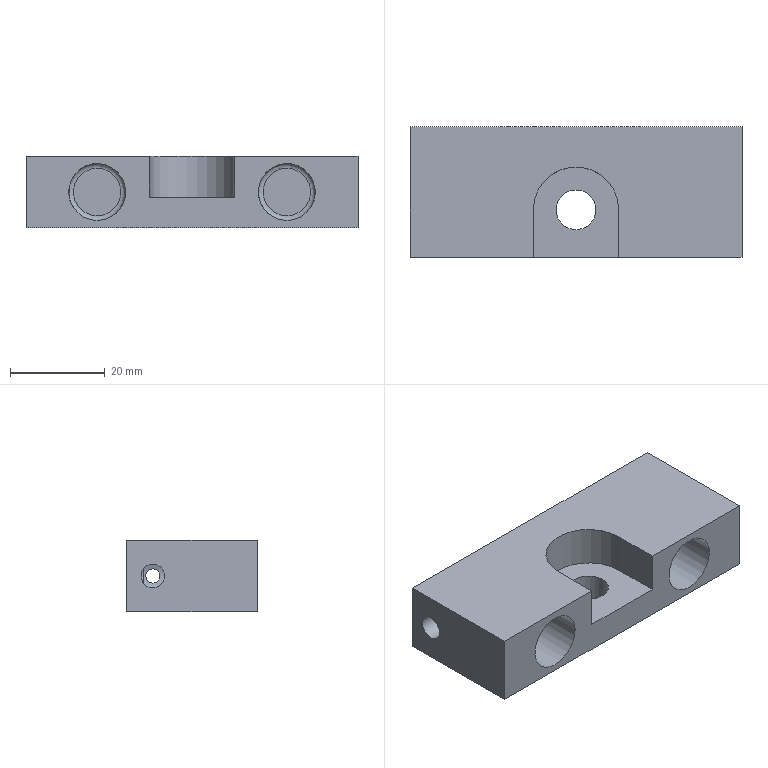Part | NX | 1 solid | 20 faces | box 70 x 27.5 x 15 mm | volume 19680 mm3 | plane 11 | cylinder 7 | torus 2 | commonest cylinder face diameters 5 x2 12 x2 3 x1 8.4 x1 18 x1
STEP:
#1=CARTESIAN_POINT('',(-25.809,10.25,-6.));
#2=VERTEX_POINT('',#1);
#3=CARTESIAN_POINT('',(-25.809,10.25,-9.));
#4=VERTEX_POINT('',#3);
#5=CARTESIAN_POINT('',(-25.809,10.25,-9.));
#6=CARTESIAN_POINT('',(-25.835,10.323,-8.902));
#7=CARTESIAN_POINT('',(-25.863,10.446,-8.704));
#8=CARTESIAN_POINT('',(-25.873,10.542,-8.508));
#9=CARTESIAN_POINT('',(-25.876,10.631,-8.268));
#10=CARTESIAN_POINT('',(-25.875,10.659,-8.178));
#11=CARTESIAN_POINT('',(-25.868,10.746,-7.791));
#12=CARTESIAN_POINT('',(-25.864,10.753,-7.504));
#13=CARTESIAN_POINT('',(-25.868,10.746,-7.206));
#14=CARTESIAN_POINT('',(-25.875,10.66,-6.826));
#15=CARTESIAN_POINT('',(-25.876,10.632,-6.733));
#16=CARTESIAN_POINT('',(-25.873,10.541,-6.491));
#17=CARTESIAN_POINT('',(-25.862,10.444,-6.293));
#18=CARTESIAN_POINT('',(-25.835,10.323,-6.098));
#19=CARTESIAN_POINT('',(-25.809,10.25,-6.));
#20=B_SPLINE_CURVE_WITH_KNOTS('',3,(#5,#6,#7,#8,#9,#10,#11,#12,#13,#14,#15,#16,#17,#18,#19),.UNSPECIFIED.,.F.,.F.,(4,1,1,1,1,1,1,1,1,1,1,1,4),(0.,0.125,0.1875,0.25,0.3125,0.375,0.5,0.625,0.6875,0.75,0.8125,0.875,1.),.UNSPECIFIED.);
#21=EDGE_CURVE('',#2,#4,#20,.F.);
#22=ORIENTED_EDGE('',*,*,#21,.F.);
#23=CARTESIAN_POINT('',(-25.809,10.25,-6.));
#24=CARTESIAN_POINT('',(-25.79,10.195,-5.926));
#25=CARTESIAN_POINT('',(-25.746,10.067,-5.766));
#26=CARTESIAN_POINT('',(-25.671,9.804,-5.539));
#27=CARTESIAN_POINT('',(-25.638,9.681,-5.445));
#28=CARTESIAN_POINT('',(-25.553,9.31,-5.222));
#29=CARTESIAN_POINT('',(-25.488,8.921,-5.075));
#30=CARTESIAN_POINT('',(-25.444,8.343,-4.977));
#31=CARTESIAN_POINT('',(-25.465,7.851,-5.021));
#32=CARTESIAN_POINT('',(-25.511,7.433,-5.127));
#33=CARTESIAN_POINT('',(-25.556,7.185,-5.234));
#34=CARTESIAN_POINT('',(-25.605,6.955,-5.356));
#35=CARTESIAN_POINT('',(-25.659,6.74,-5.506));
#36=CARTESIAN_POINT('',(-25.675,6.681,-5.549));
#37=CARTESIAN_POINT('',(-25.762,6.385,-5.817));
#38=CARTESIAN_POINT('',(-25.814,6.235,-6.008));
#39=CARTESIAN_POINT('',(-25.903,5.99,-6.404));
#40=CARTESIAN_POINT('',(-25.969,5.826,-6.822));
#41=CARTESIAN_POINT('',(-26.021,5.698,-7.504));
#42=CARTESIAN_POINT('',(-25.968,5.828,-8.185));
#43=CARTESIAN_POINT('',(-25.902,5.992,-8.602));
#44=CARTESIAN_POINT('',(-25.813,6.238,-8.997));
#45=CARTESIAN_POINT('',(-25.761,6.388,-9.186));
#46=CARTESIAN_POINT('',(-25.675,6.682,-9.451));
#47=CARTESIAN_POINT('',(-25.658,6.745,-9.498));
#48=CARTESIAN_POINT('',(-25.604,6.959,-9.646));
#49=CARTESIAN_POINT('',(-25.556,7.188,-9.768));
#50=CARTESIAN_POINT('',(-25.491,7.552,-9.921));
#51=CARTESIAN_POINT('',(-25.431,8.229,-10.052));
#52=CARTESIAN_POINT('',(-25.489,8.924,-9.922));
#53=CARTESIAN_POINT('',(-25.553,9.314,-9.777));
#54=CARTESIAN_POINT('',(-25.638,9.684,-9.553));
#55=CARTESIAN_POINT('',(-25.671,9.806,-9.46));
#56=CARTESIAN_POINT('',(-25.747,10.069,-9.231));
#57=CARTESIAN_POINT('',(-25.79,10.195,-9.074));
#58=CARTESIAN_POINT('',(-25.809,10.25,-9.));
#59=B_SPLINE_CURVE_WITH_KNOTS('',3,(#23,#24,#25,#26,#27,#28,#29,#30,#31,#32,#33,#34,#35,#36,#37,#38,#39,#40,#41,#42,#43,#44,#45,#46,#47,#48,#49,#50,#51,#52,#53,#54,#55,#56,#57,#58),.UNSPECIFIED.,.F.,.F.,(4,1,1,1,1,1,1,1,1,1,1,1,1,1,1,1,1,1,1,1,1,1,1,1,1,1,1,1,1,1,1,1,1,4),(0.,0.03125,0.04688,0.0625,0.09375,0.125,0.1875,0.2188,0.25,0.2812,0.2969,0.3125,0.3281,0.3438,0.375,0.4062,0.4375,0.5,0.5625,0.5938,0.625,0.6562,0.6719,0.6875,0.7031,0.7188,0.75,0.8125,0.875,0.9062,0.9375,0.9531,0.9688,1.),.UNSPECIFIED.);
#60=EDGE_CURVE('',#4,#2,#59,.F.);
#61=ORIENTED_EDGE('',*,*,#60,.F.);
#62=EDGE_LOOP('',(#22,#61));
#63=FACE_BOUND('',#62,.T.);
#64=CARTESIAN_POINT('',(-35.,5.75,-7.5));
#65=VERTEX_POINT('',#64);
#66=CARTESIAN_POINT('',(-35.,8.25,-7.5));
#67=DIRECTION('',(-1.,0.,0.));
#68=DIRECTION('',(0.,-1.,0.));
#69=AXIS2_PLACEMENT_3D('',#66,#67,#68);
#70=CIRCLE('',#69,2.5);
#71=EDGE_CURVE('',#65,#65,#70,.T.);
#72=ORIENTED_EDGE('',*,*,#71,.T.);
#73=EDGE_LOOP('',(#72));
#74=FACE_BOUND('',#73,.T.);
#75=CARTESIAN_POINT('',(-20.,8.25,-7.5));
#76=DIRECTION('',(-1.,0.,0.));
#77=DIRECTION('',(0.,0.,1.));
#78=AXIS2_PLACEMENT_3D('',#75,#76,#77);
#79=CYLINDRICAL_SURFACE('',#78,2.5);
#80=ADVANCED_FACE('',(#63,#74),#79,.F.);
#81=CARTESIAN_POINT('',(-14.191,8.25,-9.));
#82=VERTEX_POINT('',#81);
#83=CARTESIAN_POINT('',(-14.169,8.786,-8.915));
#84=CARTESIAN_POINT('',(-14.204,8.276,-9.053));
#85=CARTESIAN_POINT('',(-14.172,7.744,-8.926));
#86=CARTESIAN_POINT('',(-14.143,7.499,-8.807));
#87=CARTESIAN_POINT('',(-14.1,7.208,-8.604));
#88=CARTESIAN_POINT('',(-14.053,6.973,-8.305));
#89=CARTESIAN_POINT('',(-14.021,6.837,-8.041));
#90=CARTESIAN_POINT('',(-13.987,6.699,-7.532));
#91=CARTESIAN_POINT('',(-14.017,6.818,-7.007));
#92=CARTESIAN_POINT('',(-14.047,6.947,-6.743));
#93=CARTESIAN_POINT('',(-14.088,7.144,-6.46));
#94=CARTESIAN_POINT('',(-14.137,7.451,-6.219));
#95=CARTESIAN_POINT('',(-14.168,7.708,-6.088));
#96=CARTESIAN_POINT('',(-14.204,8.218,-5.948));
#97=CARTESIAN_POINT('',(-14.173,8.745,-6.07));
#98=CARTESIAN_POINT('',(-14.143,9.,-6.192));
#99=CARTESIAN_POINT('',(-14.1,9.291,-6.395));
#100=CARTESIAN_POINT('',(-14.053,9.526,-6.694));
#101=CARTESIAN_POINT('',(-14.021,9.663,-6.96));
#102=CARTESIAN_POINT('',(-13.988,9.801,-7.468));
#103=CARTESIAN_POINT('',(-14.017,9.682,-7.992));
#104=CARTESIAN_POINT('',(-14.047,9.553,-8.257));
#105=CARTESIAN_POINT('',(-14.088,9.357,-8.539));
#106=CARTESIAN_POINT('',(-14.137,9.05,-8.781));
#107=CARTESIAN_POINT('',(-14.169,8.786,-8.915));
#108=CARTESIAN_POINT('',(-14.204,8.276,-9.053));
#109=CARTESIAN_POINT('',(-14.172,7.744,-8.926));
#110=B_SPLINE_CURVE_WITH_KNOTS('',3,(#83,#84,#85,#86,#87,#88,#89,#90,#91,#92,#93,#94,#95,#96,#97,#98,#99,#100,#101,#102,#103,#104,#105,#106,#107,#108,#109),.UNSPECIFIED.,.T.,.F.,(1,1,1,1,1,1,1,1,1,1,1,1,1,1,1,1,1,1,1,1,1,1,1,1,1,1,1,1,1,1,1),(-0.1283,-0.09704,-0.06579,0.,0.05937,0.09055,0.1217,0.153,0.1842,0.2467,0.3092,0.3405,0.3717,0.403,0.4342,0.4967,0.5592,0.5905,0.6217,0.653,0.6842,0.7467,0.8092,0.8405,0.8717,0.903,0.9342,1.,1.059,1.091,1.122),.UNSPECIFIED.);
#111=EDGE_CURVE('',#82,#82,#110,.F.);
#112=ORIENTED_EDGE('',*,*,#111,.F.);
#113=EDGE_LOOP('',(#112));
#114=FACE_BOUND('',#113,.T.);
#115=CARTESIAN_POINT('',(14.191,8.25,-9.));
#116=VERTEX_POINT('',#115);
#117=CARTESIAN_POINT('',(14.169,7.714,-8.915));
#118=CARTESIAN_POINT('',(14.204,8.224,-9.053));
#119=CARTESIAN_POINT('',(14.172,8.756,-8.926));
#120=CARTESIAN_POINT('',(14.143,9.001,-8.807));
#121=CARTESIAN_POINT('',(14.1,9.292,-8.604));
#122=CARTESIAN_POINT('',(14.053,9.527,-8.305));
#123=CARTESIAN_POINT('',(14.021,9.663,-8.041));
#124=CARTESIAN_POINT('',(13.987,9.801,-7.532));
#125=CARTESIAN_POINT('',(14.017,9.682,-7.007));
#126=CARTESIAN_POINT('',(14.047,9.553,-6.743));
#127=CARTESIAN_POINT('',(14.088,9.356,-6.46));
#128=CARTESIAN_POINT('',(14.137,9.049,-6.219));
#129=CARTESIAN_POINT('',(14.168,8.792,-6.088));
#130=CARTESIAN_POINT('',(14.204,8.282,-5.948));
#131=CARTESIAN_POINT('',(14.173,7.755,-6.07));
#132=CARTESIAN_POINT('',(14.143,7.5,-6.192));
#133=CARTESIAN_POINT('',(14.1,7.209,-6.395));
#134=CARTESIAN_POINT('',(14.053,6.974,-6.694));
#135=CARTESIAN_POINT('',(14.021,6.837,-6.96));
#136=CARTESIAN_POINT('',(13.988,6.699,-7.468));
#137=CARTESIAN_POINT('',(14.017,6.818,-7.992));
#138=CARTESIAN_POINT('',(14.047,6.947,-8.257));
#139=CARTESIAN_POINT('',(14.088,7.143,-8.539));
#140=CARTESIAN_POINT('',(14.137,7.45,-8.781));
#141=CARTESIAN_POINT('',(14.169,7.714,-8.915));
#142=CARTESIAN_POINT('',(14.204,8.224,-9.053));
#143=CARTESIAN_POINT('',(14.172,8.756,-8.926));
#144=B_SPLINE_CURVE_WITH_KNOTS('',3,(#117,#118,#119,#120,#121,#122,#123,#124,#125,#126,#127,#128,#129,#130,#131,#132,#133,#134,#135,#136,#137,#138,#139,#140,#141,#142,#143),.UNSPECIFIED.,.T.,.F.,(1,1,1,1,1,1,1,1,1,1,1,1,1,1,1,1,1,1,1,1,1,1,1,1,1,1,1,1,1,1,1),(-0.1283,-0.09704,-0.06579,0.,0.05937,0.09055,0.1217,0.153,0.1842,0.2467,0.3092,0.3405,0.3717,0.403,0.4342,0.4967,0.5592,0.5905,0.6217,0.653,0.6842,0.7467,0.8092,0.8405,0.8717,0.903,0.9342,1.,1.059,1.091,1.122),.UNSPECIFIED.);
#145=EDGE_CURVE('',#116,#116,#144,.F.);
#146=ORIENTED_EDGE('',*,*,#145,.F.);
#147=EDGE_LOOP('',(#146));
#148=FACE_BOUND('',#147,.T.);
#149=CARTESIAN_POINT('',(-20.,8.25,-7.5));
#150=DIRECTION('',(1.,0.,0.));
#151=DIRECTION('',(0.,0.,-1.));
#152=AXIS2_PLACEMENT_3D('',#149,#150,#151);
#153=CYLINDRICAL_SURFACE('',#152,1.5);
#154=ADVANCED_FACE('',(#114,#148),#153,.F.);
#155=CARTESIAN_POINT('',(25.809,10.25,-9.));
#156=VERTEX_POINT('',#155);
#157=CARTESIAN_POINT('',(25.809,10.25,-6.));
#158=VERTEX_POINT('',#157);
#159=CARTESIAN_POINT('',(25.809,10.25,-6.));
#160=CARTESIAN_POINT('',(25.835,10.323,-6.098));
#161=CARTESIAN_POINT('',(25.863,10.446,-6.296));
#162=CARTESIAN_POINT('',(25.873,10.542,-6.492));
#163=CARTESIAN_POINT('',(25.876,10.631,-6.732));
#164=CARTESIAN_POINT('',(25.875,10.659,-6.822));
#165=CARTESIAN_POINT('',(25.868,10.746,-7.209));
#166=CARTESIAN_POINT('',(25.864,10.753,-7.496));
#167=CARTESIAN_POINT('',(25.868,10.746,-7.794));
#168=CARTESIAN_POINT('',(25.875,10.66,-8.174));
#169=CARTESIAN_POINT('',(25.876,10.632,-8.267));
#170=CARTESIAN_POINT('',(25.873,10.541,-8.509));
#171=CARTESIAN_POINT('',(25.862,10.444,-8.707));
#172=CARTESIAN_POINT('',(25.835,10.323,-8.902));
#173=CARTESIAN_POINT('',(25.809,10.25,-9.));
#174=B_SPLINE_CURVE_WITH_KNOTS('',3,(#159,#160,#161,#162,#163,#164,#165,#166,#167,#168,#169,#170,#171,#172,#173),.UNSPECIFIED.,.F.,.F.,(4,1,1,1,1,1,1,1,1,1,1,1,4),(0.,0.125,0.1875,0.25,0.3125,0.375,0.5,0.625,0.6875,0.75,0.8125,0.875,1.),.UNSPECIFIED.);
#175=EDGE_CURVE('',#156,#158,#174,.F.);
#176=ORIENTED_EDGE('',*,*,#175,.F.);
#177=CARTESIAN_POINT('',(25.809,10.25,-9.));
#178=CARTESIAN_POINT('',(25.79,10.195,-9.074));
#179=CARTESIAN_POINT('',(25.746,10.067,-9.234));
#180=CARTESIAN_POINT('',(25.671,9.804,-9.461));
#181=CARTESIAN_POINT('',(25.638,9.681,-9.555));
#182=CARTESIAN_POINT('',(25.553,9.31,-9.778));
#183=CARTESIAN_POINT('',(25.488,8.921,-9.925));
#184=CARTESIAN_POINT('',(25.444,8.343,-10.023));
#185=CARTESIAN_POINT('',(25.465,7.851,-9.979));
#186=CARTESIAN_POINT('',(25.511,7.433,-9.873));
#187=CARTESIAN_POINT('',(25.556,7.185,-9.766));
#188=CARTESIAN_POINT('',(25.605,6.955,-9.644));
#189=CARTESIAN_POINT('',(25.659,6.74,-9.494));
#190=CARTESIAN_POINT('',(25.675,6.681,-9.451));
#191=CARTESIAN_POINT('',(25.762,6.385,-9.183));
#192=CARTESIAN_POINT('',(25.814,6.235,-8.992));
#193=CARTESIAN_POINT('',(25.903,5.99,-8.596));
#194=CARTESIAN_POINT('',(25.969,5.826,-8.178));
#195=CARTESIAN_POINT('',(26.021,5.698,-7.496));
#196=CARTESIAN_POINT('',(25.968,5.828,-6.815));
#197=CARTESIAN_POINT('',(25.902,5.992,-6.398));
#198=CARTESIAN_POINT('',(25.813,6.238,-6.003));
#199=CARTESIAN_POINT('',(25.761,6.388,-5.814));
#200=CARTESIAN_POINT('',(25.675,6.682,-5.549));
#201=CARTESIAN_POINT('',(25.658,6.745,-5.502));
#202=CARTESIAN_POINT('',(25.604,6.959,-5.354));
#203=CARTESIAN_POINT('',(25.556,7.188,-5.232));
#204=CARTESIAN_POINT('',(25.491,7.552,-5.079));
#205=CARTESIAN_POINT('',(25.431,8.229,-4.948));
#206=CARTESIAN_POINT('',(25.489,8.924,-5.078));
#207=CARTESIAN_POINT('',(25.553,9.314,-5.223));
#208=CARTESIAN_POINT('',(25.638,9.684,-5.447));
#209=CARTESIAN_POINT('',(25.671,9.806,-5.54));
#210=CARTESIAN_POINT('',(25.747,10.069,-5.769));
#211=CARTESIAN_POINT('',(25.79,10.195,-5.926));
#212=CARTESIAN_POINT('',(25.809,10.25,-6.));
#213=B_SPLINE_CURVE_WITH_KNOTS('',3,(#177,#178,#179,#180,#181,#182,#183,#184,#185,#186,#187,#188,#189,#190,#191,#192,#193,#194,#195,#196,#197,#198,#199,#200,#201,#202,#203,#204,#205,#206,#207,#208,#209,#210,#211,#212),.UNSPECIFIED.,.F.,.F.,(4,1,1,1,1,1,1,1,1,1,1,1,1,1,1,1,1,1,1,1,1,1,1,1,1,1,1,1,1,1,1,1,1,4),(0.,0.03125,0.04688,0.0625,0.09375,0.125,0.1875,0.2188,0.25,0.2812,0.2969,0.3125,0.3281,0.3438,0.375,0.4062,0.4375,0.5,0.5625,0.5938,0.625,0.6562,0.6719,0.6875,0.7031,0.7188,0.75,0.8125,0.875,0.9062,0.9375,0.9531,0.9688,1.),.UNSPECIFIED.);
#214=EDGE_CURVE('',#158,#156,#213,.F.);
#215=ORIENTED_EDGE('',*,*,#214,.F.);
#216=EDGE_LOOP('',(#176,#215));
#217=FACE_BOUND('',#216,.T.);
#218=CARTESIAN_POINT('',(35.,10.75,-7.5));
#219=VERTEX_POINT('',#218);
#220=CARTESIAN_POINT('',(35.,8.25,-7.5));
#221=DIRECTION('',(1.,0.,0.));
#222=DIRECTION('',(0.,1.,0.));
#223=AXIS2_PLACEMENT_3D('',#220,#221,#222);
#224=CIRCLE('',#223,2.5);
#225=EDGE_CURVE('',#219,#219,#224,.T.);
#226=ORIENTED_EDGE('',*,*,#225,.T.);
#227=EDGE_LOOP('',(#226));
#228=FACE_BOUND('',#227,.T.);
#229=CARTESIAN_POINT('',(20.,8.25,-7.5));
#230=DIRECTION('',(1.,0.,0.));
#231=DIRECTION('',(0.,0.,-1.));
#232=AXIS2_PLACEMENT_3D('',#229,#230,#231);
#233=CYLINDRICAL_SURFACE('',#232,2.5);
#234=ADVANCED_FACE('',(#217,#228),#233,.F.);
#235=CARTESIAN_POINT('',(-20.,11.25,-12.5));
#236=VERTEX_POINT('',#235);
#237=CARTESIAN_POINT('',(-20.,11.25,-7.5));
#238=DIRECTION('',(0.,-1.,0.));
#239=DIRECTION('',(0.,0.,-1.));
#240=AXIS2_PLACEMENT_3D('',#237,#238,#239);
#241=CIRCLE('',#240,5.);
#242=EDGE_CURVE('',#236,#236,#241,.T.);
#243=ORIENTED_EDGE('',*,*,#242,.F.);
#244=EDGE_LOOP('',(#243));
#245=FACE_BOUND('',#244,.T.);
#246=CARTESIAN_POINT('',(-20.,10.25,-7.5));
#247=DIRECTION('',(0.,-1.,0.));
#248=DIRECTION('',(0.,0.,-1.));
#249=AXIS2_PLACEMENT_3D('',#246,#247,#248);
#250=CIRCLE('',#249,6.);
#251=EDGE_CURVE('',#4,#2,#250,.T.);
#252=ORIENTED_EDGE('',*,*,#251,.T.);
#253=ORIENTED_EDGE('',*,*,#21,.T.);
#254=EDGE_LOOP('',(#252,#253));
#255=FACE_BOUND('',#254,.T.);
#256=CARTESIAN_POINT('',(-20.,10.25,-7.5));
#257=DIRECTION('',(0.,-1.,0.));
#258=DIRECTION('',(0.,0.,-1.));
#259=AXIS2_PLACEMENT_3D('',#256,#257,#258);
#260=TOROIDAL_SURFACE('',#259,5.,1.);
#261=ADVANCED_FACE('',(#245,#255),#260,.F.);
#262=CARTESIAN_POINT('',(20.,11.25,-12.5));
#263=VERTEX_POINT('',#262);
#264=CARTESIAN_POINT('',(20.,11.25,-7.5));
#265=DIRECTION('',(0.,-1.,0.));
#266=DIRECTION('',(0.,0.,-1.));
#267=AXIS2_PLACEMENT_3D('',#264,#265,#266);
#268=CIRCLE('',#267,5.);
#269=EDGE_CURVE('',#263,#263,#268,.T.);
#270=ORIENTED_EDGE('',*,*,#269,.F.);
#271=EDGE_LOOP('',(#270));
#272=FACE_BOUND('',#271,.T.);
#273=CARTESIAN_POINT('',(20.,10.25,-7.5));
#274=DIRECTION('',(0.,-1.,0.));
#275=DIRECTION('',(0.,0.,-1.));
#276=AXIS2_PLACEMENT_3D('',#273,#274,#275);
#277=CIRCLE('',#276,6.);
#278=EDGE_CURVE('',#158,#156,#277,.T.);
#279=ORIENTED_EDGE('',*,*,#278,.T.);
#280=ORIENTED_EDGE('',*,*,#175,.T.);
#281=EDGE_LOOP('',(#279,#280));
#282=FACE_BOUND('',#281,.T.);
#283=CARTESIAN_POINT('',(20.,10.25,-7.5));
#284=DIRECTION('',(0.,-1.,0.));
#285=DIRECTION('',(0.,0.,-1.));
#286=AXIS2_PLACEMENT_3D('',#283,#284,#285);
#287=TOROIDAL_SURFACE('',#286,5.,1.);
#288=ADVANCED_FACE('',(#272,#282),#287,.F.);
#289=ORIENTED_EDGE('',*,*,#269,.T.);
#290=EDGE_LOOP('',(#289));
#291=FACE_BOUND('',#290,.T.);
#292=CARTESIAN_POINT('',(20.,11.25,-7.5));
#293=DIRECTION('',(0.,-1.,0.));
#294=DIRECTION('',(0.,0.,-1.));
#295=AXIS2_PLACEMENT_3D('',#292,#293,#294);
#296=PLANE('',#295);
#297=ADVANCED_FACE('',(#291),#296,.T.);
#298=ORIENTED_EDGE('',*,*,#145,.T.);
#299=EDGE_LOOP('',(#298));
#300=FACE_BOUND('',#299,.T.);
#301=CARTESIAN_POINT('',(14.,-13.75,-7.5));
#302=VERTEX_POINT('',#301);
#303=CARTESIAN_POINT('',(20.,-13.75,-7.5));
#304=DIRECTION('',(0.,1.,0.));
#305=DIRECTION('',(-1.,0.,0.));
#306=AXIS2_PLACEMENT_3D('',#303,#304,#305);
#307=CIRCLE('',#306,6.);
#308=EDGE_CURVE('',#302,#302,#307,.F.);
#309=ORIENTED_EDGE('',*,*,#308,.T.);
#310=EDGE_LOOP('',(#309));
#311=FACE_BOUND('',#310,.T.);
#312=ORIENTED_EDGE('',*,*,#278,.F.);
#313=ORIENTED_EDGE('',*,*,#214,.T.);
#314=EDGE_LOOP('',(#312,#313));
#315=FACE_BOUND('',#314,.T.);
#316=CARTESIAN_POINT('',(20.,11.25,-7.5));
#317=DIRECTION('',(0.,-1.,0.));
#318=DIRECTION('',(0.,0.,-1.));
#319=AXIS2_PLACEMENT_3D('',#316,#317,#318);
#320=CYLINDRICAL_SURFACE('',#319,6.);
#321=ADVANCED_FACE('',(#300,#311,#315),#320,.F.);
#322=ORIENTED_EDGE('',*,*,#242,.T.);
#323=EDGE_LOOP('',(#322));
#324=FACE_BOUND('',#323,.T.);
#325=CARTESIAN_POINT('',(-20.,11.25,-7.5));
#326=DIRECTION('',(0.,-1.,0.));
#327=DIRECTION('',(0.,0.,-1.));
#328=AXIS2_PLACEMENT_3D('',#325,#326,#327);
#329=PLANE('',#328);
#330=ADVANCED_FACE('',(#324),#329,.T.);
#331=ORIENTED_EDGE('',*,*,#111,.T.);
#332=EDGE_LOOP('',(#331));
#333=FACE_BOUND('',#332,.T.);
#334=CARTESIAN_POINT('',(-14.,-13.75,-7.5));
#335=VERTEX_POINT('',#334);
#336=CARTESIAN_POINT('',(-20.,-13.75,-7.5));
#337=DIRECTION('',(0.,-1.,0.));
#338=DIRECTION('',(1.,0.,0.));
#339=AXIS2_PLACEMENT_3D('',#336,#337,#338);
#340=CIRCLE('',#339,6.);
#341=EDGE_CURVE('',#335,#335,#340,.T.);
#342=ORIENTED_EDGE('',*,*,#341,.T.);
#343=EDGE_LOOP('',(#342));
#344=FACE_BOUND('',#343,.T.);
#345=ORIENTED_EDGE('',*,*,#251,.F.);
#346=ORIENTED_EDGE('',*,*,#60,.T.);
#347=EDGE_LOOP('',(#345,#346));
#348=FACE_BOUND('',#347,.T.);
#349=CARTESIAN_POINT('',(-20.,11.25,-7.5));
#350=DIRECTION('',(0.,-1.,0.));
#351=DIRECTION('',(0.,0.,-1.));
#352=AXIS2_PLACEMENT_3D('',#349,#350,#351);
#353=CYLINDRICAL_SURFACE('',#352,6.);
#354=ADVANCED_FACE('',(#333,#344,#348),#353,.F.);
#355=CARTESIAN_POINT('',(4.2,-3.75,-15.));
#356=VERTEX_POINT('',#355);
#357=CARTESIAN_POINT('',(0.,-3.75,-15.));
#358=DIRECTION('',(0.,0.,1.));
#359=DIRECTION('',(1.,0.,0.));
#360=AXIS2_PLACEMENT_3D('',#357,#358,#359);
#361=CIRCLE('',#360,4.2);
#362=EDGE_CURVE('',#356,#356,#361,.T.);
#363=ORIENTED_EDGE('',*,*,#362,.F.);
#364=EDGE_LOOP('',(#363));
#365=FACE_BOUND('',#364,.T.);
#366=CARTESIAN_POINT('',(4.2,-3.75,-8.6));
#367=VERTEX_POINT('',#366);
#368=CARTESIAN_POINT('',(0.,-3.75,-8.6));
#369=DIRECTION('',(0.,0.,1.));
#370=DIRECTION('',(1.,0.,0.));
#371=AXIS2_PLACEMENT_3D('',#368,#369,#370);
#372=CIRCLE('',#371,4.2);
#373=EDGE_CURVE('',#367,#367,#372,.T.);
#374=ORIENTED_EDGE('',*,*,#373,.T.);
#375=EDGE_LOOP('',(#374));
#376=FACE_BOUND('',#375,.T.);
#377=CARTESIAN_POINT('',(0.,-3.75,-15.));
#378=DIRECTION('',(0.,0.,1.));
#379=DIRECTION('',(1.,0.,0.));
#380=AXIS2_PLACEMENT_3D('',#377,#378,#379);
#381=CYLINDRICAL_SURFACE('',#380,4.2);
#382=ADVANCED_FACE('',(#365,#376),#381,.F.);
#383=ORIENTED_EDGE('',*,*,#373,.F.);
#384=EDGE_LOOP('',(#383));
#385=FACE_BOUND('',#384,.T.);
#386=CARTESIAN_POINT('',(9.,-13.75,-8.6));
#387=VERTEX_POINT('',#386);
#388=CARTESIAN_POINT('',(-9.,-13.75,-8.6));
#389=VERTEX_POINT('',#388);
#390=CARTESIAN_POINT('',(0.,-13.75,-8.6));
#391=DIRECTION('',(-1.,0.,0.));
#392=VECTOR('',#391,1000.);
#393=LINE('',#390,#392);
#394=EDGE_CURVE('',#387,#389,#393,.T.);
#395=ORIENTED_EDGE('',*,*,#394,.F.);
#396=CARTESIAN_POINT('',(9.,-3.75,-8.6));
#397=VERTEX_POINT('',#396);
#398=CARTESIAN_POINT('',(9.,-3.75,-8.6));
#399=DIRECTION('',(0.,-1.,0.));
#400=VECTOR('',#399,1000.);
#401=LINE('',#398,#400);
#402=EDGE_CURVE('',#397,#387,#401,.T.);
#403=ORIENTED_EDGE('',*,*,#402,.F.);
#404=CARTESIAN_POINT('',(-9.,-3.75,-8.6));
#405=VERTEX_POINT('',#404);
#406=CARTESIAN_POINT('',(0.,-3.75,-8.6));
#407=DIRECTION('',(0.,0.,1.));
#408=DIRECTION('',(1.,0.,0.));
#409=AXIS2_PLACEMENT_3D('',#406,#407,#408);
#410=CIRCLE('',#409,9.);
#411=EDGE_CURVE('',#397,#405,#410,.T.);
#412=ORIENTED_EDGE('',*,*,#411,.T.);
#413=CARTESIAN_POINT('',(-9.,-13.75,-8.6));
#414=DIRECTION('',(0.,1.,0.));
#415=VECTOR('',#414,1000.);
#416=LINE('',#413,#415);
#417=EDGE_CURVE('',#389,#405,#416,.T.);
#418=ORIENTED_EDGE('',*,*,#417,.F.);
#419=EDGE_LOOP('',(#395,#403,#412,#418));
#420=FACE_BOUND('',#419,.T.);
#421=CARTESIAN_POINT('',(0.,-3.75,-8.6));
#422=DIRECTION('',(0.,0.,1.));
#423=DIRECTION('',(1.,0.,0.));
#424=AXIS2_PLACEMENT_3D('',#421,#422,#423);
#425=PLANE('',#424);
#426=ADVANCED_FACE('',(#385,#420),#425,.T.);
#427=CARTESIAN_POINT('',(9.,-3.75,0.));
#428=VERTEX_POINT('',#427);
#429=CARTESIAN_POINT('',(9.,-13.75,0.));
#430=VERTEX_POINT('',#429);
#431=CARTESIAN_POINT('',(9.,-3.75,0.));
#432=DIRECTION('',(0.,-1.,0.));
#433=VECTOR('',#432,1000.);
#434=LINE('',#431,#433);
#435=EDGE_CURVE('',#428,#430,#434,.T.);
#436=ORIENTED_EDGE('',*,*,#435,.F.);
#437=CARTESIAN_POINT('',(9.,-3.75,-8.6));
#438=DIRECTION('',(0.,0.,1.));
#439=VECTOR('',#438,1000.);
#440=LINE('',#437,#439);
#441=EDGE_CURVE('',#397,#428,#440,.T.);
#442=ORIENTED_EDGE('',*,*,#441,.F.);
#443=ORIENTED_EDGE('',*,*,#402,.T.);
#444=CARTESIAN_POINT('',(9.,-13.75,-15.));
#445=DIRECTION('',(0.,0.,1.));
#446=VECTOR('',#445,1000.);
#447=LINE('',#444,#446);
#448=EDGE_CURVE('',#387,#430,#447,.T.);
#449=ORIENTED_EDGE('',*,*,#448,.T.);
#450=EDGE_LOOP('',(#436,#442,#443,#449));
#451=FACE_BOUND('',#450,.T.);
#452=CARTESIAN_POINT('',(9.,-3.75,-8.6));
#453=DIRECTION('',(-1.,0.,0.));
#454=DIRECTION('',(0.,0.,1.));
#455=AXIS2_PLACEMENT_3D('',#452,#453,#454);
#456=PLANE('',#455);
#457=ADVANCED_FACE('',(#451),#456,.T.);
#458=CARTESIAN_POINT('',(-9.,-3.75,0.));
#459=VERTEX_POINT('',#458);
#460=CARTESIAN_POINT('',(0.,-3.75,0.));
#461=DIRECTION('',(0.,0.,1.));
#462=DIRECTION('',(1.,0.,0.));
#463=AXIS2_PLACEMENT_3D('',#460,#461,#462);
#464=CIRCLE('',#463,9.);
#465=EDGE_CURVE('',#428,#459,#464,.T.);
#466=ORIENTED_EDGE('',*,*,#465,.T.);
#467=CARTESIAN_POINT('',(-9.,-3.75,-8.6));
#468=DIRECTION('',(0.,0.,1.));
#469=VECTOR('',#468,1000.);
#470=LINE('',#467,#469);
#471=EDGE_CURVE('',#405,#459,#470,.T.);
#472=ORIENTED_EDGE('',*,*,#471,.F.);
#473=ORIENTED_EDGE('',*,*,#411,.F.);
#474=ORIENTED_EDGE('',*,*,#441,.T.);
#475=EDGE_LOOP('',(#466,#472,#473,#474));
#476=FACE_BOUND('',#475,.T.);
#477=CARTESIAN_POINT('',(0.,-3.75,-8.6));
#478=DIRECTION('',(0.,0.,1.));
#479=DIRECTION('',(1.,0.,0.));
#480=AXIS2_PLACEMENT_3D('',#477,#478,#479);
#481=CYLINDRICAL_SURFACE('',#480,9.);
#482=ADVANCED_FACE('',(#476),#481,.F.);
#483=CARTESIAN_POINT('',(-9.,-13.75,0.));
#484=VERTEX_POINT('',#483);
#485=CARTESIAN_POINT('',(-9.,-13.75,0.));
#486=DIRECTION('',(0.,1.,0.));
#487=VECTOR('',#486,1000.);
#488=LINE('',#485,#487);
#489=EDGE_CURVE('',#484,#459,#488,.T.);
#490=ORIENTED_EDGE('',*,*,#489,.F.);
#491=CARTESIAN_POINT('',(-9.,-13.75,-8.6));
#492=DIRECTION('',(0.,0.,1.));
#493=VECTOR('',#492,1000.);
#494=LINE('',#491,#493);
#495=EDGE_CURVE('',#389,#484,#494,.T.);
#496=ORIENTED_EDGE('',*,*,#495,.F.);
#497=ORIENTED_EDGE('',*,*,#417,.T.);
#498=ORIENTED_EDGE('',*,*,#471,.T.);
#499=EDGE_LOOP('',(#490,#496,#497,#498));
#500=FACE_BOUND('',#499,.T.);
#501=CARTESIAN_POINT('',(-9.,-13.75,-8.6));
#502=DIRECTION('',(1.,0.,0.));
#503=DIRECTION('',(0.,0.,-1.));
#504=AXIS2_PLACEMENT_3D('',#501,#502,#503);
#505=PLANE('',#504);
#506=ADVANCED_FACE('',(#500),#505,.T.);
#507=ORIENTED_EDGE('',*,*,#362,.T.);
#508=EDGE_LOOP('',(#507));
#509=FACE_BOUND('',#508,.T.);
#510=CARTESIAN_POINT('',(35.,13.75,-15.));
#511=VERTEX_POINT('',#510);
#512=CARTESIAN_POINT('',(35.,-13.75,-15.));
#513=VERTEX_POINT('',#512);
#514=CARTESIAN_POINT('',(35.,13.75,-15.));
#515=DIRECTION('',(0.,-1.,0.));
#516=VECTOR('',#515,1000.);
#517=LINE('',#514,#516);
#518=EDGE_CURVE('',#511,#513,#517,.T.);
#519=ORIENTED_EDGE('',*,*,#518,.T.);
#520=CARTESIAN_POINT('',(-35.,-13.75,-15.));
#521=VERTEX_POINT('',#520);
#522=CARTESIAN_POINT('',(-9.,-13.75,-15.));
#523=DIRECTION('',(-1.,0.,0.));
#524=VECTOR('',#523,1000.);
#525=LINE('',#522,#524);
#526=EDGE_CURVE('',#513,#521,#525,.T.);
#527=ORIENTED_EDGE('',*,*,#526,.T.);
#528=CARTESIAN_POINT('',(-35.,13.75,-15.));
#529=VERTEX_POINT('',#528);
#530=CARTESIAN_POINT('',(-35.,-13.75,-15.));
#531=DIRECTION('',(0.,1.,0.));
#532=VECTOR('',#531,1000.);
#533=LINE('',#530,#532);
#534=EDGE_CURVE('',#521,#529,#533,.T.);
#535=ORIENTED_EDGE('',*,*,#534,.T.);
#536=CARTESIAN_POINT('',(-35.,13.75,-15.));
#537=DIRECTION('',(1.,0.,0.));
#538=VECTOR('',#537,1000.);
#539=LINE('',#536,#538);
#540=EDGE_CURVE('',#529,#511,#539,.T.);
#541=ORIENTED_EDGE('',*,*,#540,.T.);
#542=EDGE_LOOP('',(#519,#527,#535,#541));
#543=FACE_BOUND('',#542,.T.);
#544=CARTESIAN_POINT('',(0.,0.,-15.));
#545=DIRECTION('',(0.,0.,-1.));
#546=DIRECTION('',(-1.,0.,0.));
#547=AXIS2_PLACEMENT_3D('',#544,#545,#546);
#548=PLANE('',#547);
#549=ADVANCED_FACE('',(#509,#543),#548,.T.);
#550=ORIENTED_EDGE('',*,*,#225,.F.);
#551=EDGE_LOOP('',(#550));
#552=FACE_BOUND('',#551,.T.);
#553=CARTESIAN_POINT('',(35.,13.75,0.));
#554=VERTEX_POINT('',#553);
#555=CARTESIAN_POINT('',(35.,-13.75,0.));
#556=VERTEX_POINT('',#555);
#557=CARTESIAN_POINT('',(35.,13.75,0.));
#558=DIRECTION('',(0.,-1.,0.));
#559=VECTOR('',#558,1000.);
#560=LINE('',#557,#559);
#561=EDGE_CURVE('',#554,#556,#560,.T.);
#562=ORIENTED_EDGE('',*,*,#561,.T.);
#563=CARTESIAN_POINT('',(35.,-13.75,-15.));
#564=DIRECTION('',(0.,0.,1.));
#565=VECTOR('',#564,1000.);
#566=LINE('',#563,#565);
#567=EDGE_CURVE('',#513,#556,#566,.T.);
#568=ORIENTED_EDGE('',*,*,#567,.F.);
#569=ORIENTED_EDGE('',*,*,#518,.F.);
#570=CARTESIAN_POINT('',(35.,13.75,-15.));
#571=DIRECTION('',(0.,0.,1.));
#572=VECTOR('',#571,1000.);
#573=LINE('',#570,#572);
#574=EDGE_CURVE('',#511,#554,#573,.T.);
#575=ORIENTED_EDGE('',*,*,#574,.T.);
#576=EDGE_LOOP('',(#562,#568,#569,#575));
#577=FACE_BOUND('',#576,.T.);
#578=CARTESIAN_POINT('',(35.,13.75,-15.));
#579=DIRECTION('',(-1.,0.,0.));
#580=DIRECTION('',(0.,0.,1.));
#581=AXIS2_PLACEMENT_3D('',#578,#579,#580);
#582=PLANE('',#581);
#583=ADVANCED_FACE('',(#552,#577),#582,.F.);
#584=CARTESIAN_POINT('',(-35.,13.75,0.));
#585=VERTEX_POINT('',#584);
#586=CARTESIAN_POINT('',(-35.,13.75,0.));
#587=DIRECTION('',(1.,0.,0.));
#588=VECTOR('',#587,1000.);
#589=LINE('',#586,#588);
#590=EDGE_CURVE('',#585,#554,#589,.T.);
#591=ORIENTED_EDGE('',*,*,#590,.T.);
#592=ORIENTED_EDGE('',*,*,#574,.F.);
#593=ORIENTED_EDGE('',*,*,#540,.F.);
#594=CARTESIAN_POINT('',(-35.,13.75,-15.));
#595=DIRECTION('',(0.,0.,1.));
#596=VECTOR('',#595,1000.);
#597=LINE('',#594,#596);
#598=EDGE_CURVE('',#529,#585,#597,.T.);
#599=ORIENTED_EDGE('',*,*,#598,.T.);
#600=EDGE_LOOP('',(#591,#592,#593,#599));
#601=FACE_BOUND('',#600,.T.);
#602=CARTESIAN_POINT('',(-35.,13.75,-15.));
#603=DIRECTION('',(0.,-1.,0.));
#604=DIRECTION('',(0.,0.,-1.));
#605=AXIS2_PLACEMENT_3D('',#602,#603,#604);
#606=PLANE('',#605);
#607=ADVANCED_FACE('',(#601),#606,.F.);
#608=ORIENTED_EDGE('',*,*,#71,.F.);
#609=EDGE_LOOP('',(#608));
#610=FACE_BOUND('',#609,.T.);
#611=CARTESIAN_POINT('',(-35.,-13.75,0.));
#612=VERTEX_POINT('',#611);
#613=CARTESIAN_POINT('',(-35.,-13.75,0.));
#614=DIRECTION('',(0.,1.,0.));
#615=VECTOR('',#614,1000.);
#616=LINE('',#613,#615);
#617=EDGE_CURVE('',#612,#585,#616,.T.);
#618=ORIENTED_EDGE('',*,*,#617,.T.);
#619=ORIENTED_EDGE('',*,*,#598,.F.);
#620=ORIENTED_EDGE('',*,*,#534,.F.);
#621=CARTESIAN_POINT('',(-35.,-13.75,-15.));
#622=DIRECTION('',(0.,0.,1.));
#623=VECTOR('',#622,1000.);
#624=LINE('',#621,#623);
#625=EDGE_CURVE('',#521,#612,#624,.T.);
#626=ORIENTED_EDGE('',*,*,#625,.T.);
#627=EDGE_LOOP('',(#618,#619,#620,#626));
#628=FACE_BOUND('',#627,.T.);
#629=CARTESIAN_POINT('',(-35.,-13.75,-15.));
#630=DIRECTION('',(1.,0.,0.));
#631=DIRECTION('',(0.,0.,-1.));
#632=AXIS2_PLACEMENT_3D('',#629,#630,#631);
#633=PLANE('',#632);
#634=ADVANCED_FACE('',(#610,#628),#633,.F.);
#635=ORIENTED_EDGE('',*,*,#489,.T.);
#636=ORIENTED_EDGE('',*,*,#465,.F.);
#637=ORIENTED_EDGE('',*,*,#435,.T.);
#638=CARTESIAN_POINT('',(-9.,-13.75,0.));
#639=DIRECTION('',(-1.,0.,0.));
#640=VECTOR('',#639,1000.);
#641=LINE('',#638,#640);
#642=EDGE_CURVE('',#556,#430,#641,.T.);
#643=ORIENTED_EDGE('',*,*,#642,.F.);
#644=ORIENTED_EDGE('',*,*,#561,.F.);
#645=ORIENTED_EDGE('',*,*,#590,.F.);
#646=ORIENTED_EDGE('',*,*,#617,.F.);
#647=CARTESIAN_POINT('',(-9.,-13.75,0.));
#648=DIRECTION('',(-1.,0.,0.));
#649=VECTOR('',#648,1000.);
#650=LINE('',#647,#649);
#651=EDGE_CURVE('',#484,#612,#650,.T.);
#652=ORIENTED_EDGE('',*,*,#651,.F.);
#653=EDGE_LOOP('',(#635,#636,#637,#643,#644,#645,#646,#652));
#654=FACE_BOUND('',#653,.T.);
#655=CARTESIAN_POINT('',(0.,0.,0.));
#656=DIRECTION('',(0.,0.,-1.));
#657=DIRECTION('',(-1.,0.,0.));
#658=AXIS2_PLACEMENT_3D('',#655,#656,#657);
#659=PLANE('',#658);
#660=ADVANCED_FACE('',(#654),#659,.F.);
#661=ORIENTED_EDGE('',*,*,#394,.T.);
#662=ORIENTED_EDGE('',*,*,#495,.T.);
#663=ORIENTED_EDGE('',*,*,#651,.T.);
#664=ORIENTED_EDGE('',*,*,#625,.F.);
#665=ORIENTED_EDGE('',*,*,#526,.F.);
#666=ORIENTED_EDGE('',*,*,#567,.T.);
#667=ORIENTED_EDGE('',*,*,#642,.T.);
#668=ORIENTED_EDGE('',*,*,#448,.F.);
#669=EDGE_LOOP('',(#661,#662,#663,#664,#665,#666,#667,#668));
#670=FACE_BOUND('',#669,.T.);
#671=ORIENTED_EDGE('',*,*,#308,.F.);
#672=EDGE_LOOP('',(#671));
#673=FACE_BOUND('',#672,.T.);
#674=ORIENTED_EDGE('',*,*,#341,.F.);
#675=EDGE_LOOP('',(#674));
#676=FACE_BOUND('',#675,.T.);
#677=CARTESIAN_POINT('',(-9.,-13.75,-15.));
#678=DIRECTION('',(0.,1.,0.));
#679=DIRECTION('',(-1.,0.,0.));
#680=AXIS2_PLACEMENT_3D('',#677,#678,#679);
#681=PLANE('',#680);
#682=ADVANCED_FACE('',(#670,#673,#676),#681,.F.);
#683=CLOSED_SHELL('',(#80,#154,#234,#261,#288,#297,#321,#330,#354,#382,#426,#457,#482,#506,#549,#583,#607,#634,#660,#682));
#684=MANIFOLD_SOLID_BREP('',#683);
#685=(LENGTH_UNIT()NAMED_UNIT(*)SI_UNIT(.MILLI.,.METRE.));
#686=UNCERTAINTY_MEASURE_WITH_UNIT(LENGTH_MEASURE(0.0508),#685,'','');
#687=(NAMED_UNIT(*)PLANE_ANGLE_UNIT()SI_UNIT($,.RADIAN.));
#688=(NAMED_UNIT(*)SI_UNIT($,.STERADIAN.)SOLID_ANGLE_UNIT());
#689=(GEOMETRIC_REPRESENTATION_CONTEXT(3)GLOBAL_UNCERTAINTY_ASSIGNED_CONTEXT((#686))GLOBAL_UNIT_ASSIGNED_CONTEXT((#685,#687,#688))REPRESENTATION_CONTEXT('',''));
#690=ADVANCED_BREP_SHAPE_REPRESENTATION('',(#684),#689);